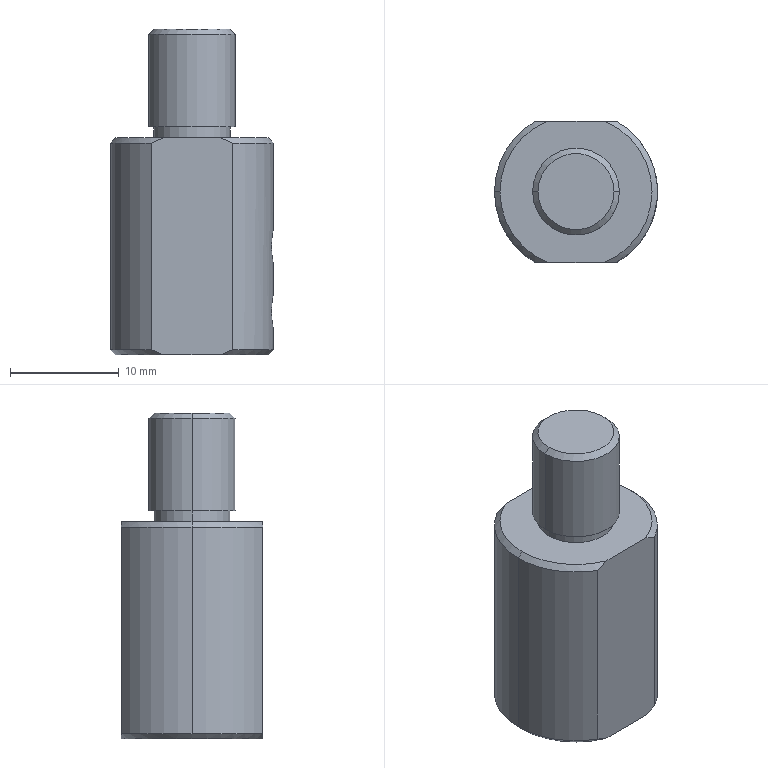Part | SolidWorks | features ICE 4, Chamfer 1, Extrusion 1, HoleWzd 1 | 1 solid | 32 faces | box 15 x 13 x 30 mm | volume 3613 mm3 | cylinder 13 | plane 11 | cone 8 | commonest cylinder face diameters 3.3 x4 15 x3 3 x2 7 x2 8 x2
STEP:
#1=CARTESIAN_POINT('',(7.5,0.,2.35));
#2=VERTEX_POINT('',#1);
#3=CARTESIAN_POINT('',(7.5,0.,5.65));
#4=VERTEX_POINT('',#3);
#5=CARTESIAN_POINT('',(7.5,0.,2.35));
#6=CARTESIAN_POINT('',(7.5,-0.2157,2.35));
#7=CARTESIAN_POINT('',(7.49,-0.4334,2.393));
#8=CARTESIAN_POINT('',(7.465,-0.7314,2.517));
#9=CARTESIAN_POINT('',(7.455,-0.8278,2.569));
#10=CARTESIAN_POINT('',(7.433,-1.007,2.689));
#11=CARTESIAN_POINT('',(7.421,-1.09,2.757));
#12=CARTESIAN_POINT('',(7.397,-1.242,2.909));
#13=CARTESIAN_POINT('',(7.385,-1.312,2.993));
#14=CARTESIAN_POINT('',(7.362,-1.431,3.172));
#15=CARTESIAN_POINT('',(7.352,-1.482,3.266));
#16=CARTESIAN_POINT('',(7.326,-1.607,3.567));
#17=CARTESIAN_POINT('',(7.316,-1.65,3.782));
#18=CARTESIAN_POINT('',(7.316,-1.65,4.108));
#19=CARTESIAN_POINT('',(7.319,-1.639,4.216));
#20=CARTESIAN_POINT('',(7.328,-1.597,4.427));
#21=CARTESIAN_POINT('',(7.335,-1.565,4.532));
#22=CARTESIAN_POINT('',(7.361,-1.442,4.831));
#23=CARTESIAN_POINT('',(7.385,-1.319,5.014));
#24=CARTESIAN_POINT('',(7.432,-1.016,5.318));
#25=CARTESIAN_POINT('',(7.456,-0.8326,5.441));
#26=CARTESIAN_POINT('',(7.482,-0.5349,5.565));
#27=CARTESIAN_POINT('',(7.488,-0.43,5.597));
#28=CARTESIAN_POINT('',(7.498,-0.2172,5.639));
#29=CARTESIAN_POINT('',(7.5,-0.1094,5.65));
#30=CARTESIAN_POINT('',(7.5,0.,5.65));
#31=B_SPLINE_CURVE_WITH_KNOTS('',3,(#5,#6,#7,#8,#9,#10,#11,#12,#13,#14,#15,#16,#17,#18,#19,#20,#21,#22,#23,#24,#25,#26,#27,#28,#29,#30),.UNSPECIFIED.,.F.,.F.,(4,2,2,2,2,2,2,2,2,2,2,2,4),(0.005175,0.005821,0.006144,0.006468,0.006791,0.007114,0.007761,0.008084,0.008408,0.009054,0.009701,0.01002,0.01035),.UNSPECIFIED.);
#32=EDGE_CURVE('',#2,#4,#31,.T.);
#33=ORIENTED_EDGE('',*,*,#32,.F.);
#34=CARTESIAN_POINT('',(1.5,0.,2.35));
#35=VERTEX_POINT('',#34);
#36=CARTESIAN_POINT('',(0.,0.,2.35));
#37=DIRECTION('',(-1.,0.,0.));
#38=VECTOR('',#37,1000.);
#39=LINE('',#36,#38);
#40=EDGE_CURVE('',#2,#35,#39,.T.);
#41=ORIENTED_EDGE('',*,*,#40,.T.);
#42=CARTESIAN_POINT('',(0.,-1.5,3.313));
#43=VERTEX_POINT('',#42);
#44=CARTESIAN_POINT('',(0.,-1.5,3.313));
#45=CARTESIAN_POINT('',(0.1094,-1.5,3.313));
#46=CARTESIAN_POINT('',(0.2147,-1.488,3.285));
#47=CARTESIAN_POINT('',(0.4105,-1.446,3.204));
#48=CARTESIAN_POINT('',(0.5002,-1.417,3.152));
#49=CARTESIAN_POINT('',(0.7569,-1.308,2.986));
#50=CARTESIAN_POINT('',(0.9049,-1.21,2.866));
#51=CARTESIAN_POINT('',(1.172,-0.9546,2.644));
#52=CARTESIAN_POINT('',(1.286,-0.798,2.542));
#53=CARTESIAN_POINT('',(1.411,-0.5202,2.431));
#54=CARTESIAN_POINT('',(1.443,-0.4223,2.401));
#55=CARTESIAN_POINT('',(1.488,-0.2144,2.361));
#56=CARTESIAN_POINT('',(1.5,-0.1072,2.35));
#57=CARTESIAN_POINT('',(1.5,0.,2.35));
#58=B_SPLINE_CURVE_WITH_KNOTS('',3,(#44,#45,#46,#47,#48,#49,#50,#51,#52,#53,#54,#55,#56,#57),.UNSPECIFIED.,.F.,.F.,(4,2,2,2,2,2,4),(0.,0.000322,0.000644,0.001288,0.001932,0.002254,0.002576),.UNSPECIFIED.);
#59=EDGE_CURVE('',#43,#35,#58,.T.);
#60=ORIENTED_EDGE('',*,*,#59,.F.);
#61=CARTESIAN_POINT('',(0.,-1.5,4.687));
#62=VERTEX_POINT('',#61);
#63=CARTESIAN_POINT('',(0.,0.,4.));
#64=DIRECTION('',(-1.,0.,0.));
#65=DIRECTION('',(0.,0.,1.));
#66=AXIS2_PLACEMENT_3D('',#63,#64,#65);
#67=CIRCLE('',#66,1.65);
#68=EDGE_CURVE('',#43,#62,#67,.T.);
#69=ORIENTED_EDGE('',*,*,#68,.T.);
#70=CARTESIAN_POINT('',(1.5,0.,5.65));
#71=VERTEX_POINT('',#70);
#72=CARTESIAN_POINT('',(1.5,0.,5.65));
#73=CARTESIAN_POINT('',(1.5,-0.107,5.65));
#74=CARTESIAN_POINT('',(1.488,-0.2158,5.639));
#75=CARTESIAN_POINT('',(1.443,-0.4216,5.599));
#76=CARTESIAN_POINT('',(1.41,-0.5214,5.569));
#77=CARTESIAN_POINT('',(1.286,-0.7979,5.458));
#78=CARTESIAN_POINT('',(1.171,-0.9551,5.356));
#79=CARTESIAN_POINT('',(0.9067,-1.209,5.135));
#80=CARTESIAN_POINT('',(0.7555,-1.309,5.013));
#81=CARTESIAN_POINT('',(0.5018,-1.417,4.849));
#82=CARTESIAN_POINT('',(0.4108,-1.446,4.796));
#83=CARTESIAN_POINT('',(0.2156,-1.488,4.715));
#84=CARTESIAN_POINT('',(0.1091,-1.5,4.687));
#85=CARTESIAN_POINT('',(0.,-1.5,4.687));
#86=B_SPLINE_CURVE_WITH_KNOTS('',3,(#72,#73,#74,#75,#76,#77,#78,#79,#80,#81,#82,#83,#84,#85),.UNSPECIFIED.,.F.,.F.,(4,2,2,2,2,2,4),(0.002576,0.002897,0.003219,0.003861,0.004504,0.004825,0.005146),.UNSPECIFIED.);
#87=EDGE_CURVE('',#71,#62,#86,.T.);
#88=ORIENTED_EDGE('',*,*,#87,.F.);
#89=CARTESIAN_POINT('',(0.,0.,5.65));
#90=DIRECTION('',(-1.,0.,0.));
#91=VECTOR('',#90,1000.);
#92=LINE('',#89,#91);
#93=EDGE_CURVE('',#4,#71,#92,.T.);
#94=ORIENTED_EDGE('',*,*,#93,.F.);
#95=EDGE_LOOP('',(#33,#41,#60,#69,#88,#94));
#96=FACE_OUTER_BOUND('',#95,.T.);
#97=CARTESIAN_POINT('',(0.,0.,4.));
#98=DIRECTION('',(-1.,0.,0.));
#99=DIRECTION('',(0.,0.,1.));
#100=AXIS2_PLACEMENT_3D('',#97,#98,#99);
#101=CYLINDRICAL_SURFACE('',#100,1.65);
#102=ADVANCED_FACE('',(#96),#101,.F.);
#103=CARTESIAN_POINT('',(7.5,0.,8.35));
#104=VERTEX_POINT('',#103);
#105=CARTESIAN_POINT('',(7.5,0.,11.65));
#106=VERTEX_POINT('',#105);
#107=CARTESIAN_POINT('',(7.5,0.,8.35));
#108=CARTESIAN_POINT('',(7.5,-0.2157,8.35));
#109=CARTESIAN_POINT('',(7.49,-0.4334,8.393));
#110=CARTESIAN_POINT('',(7.465,-0.7314,8.517));
#111=CARTESIAN_POINT('',(7.455,-0.8278,8.569));
#112=CARTESIAN_POINT('',(7.433,-1.007,8.689));
#113=CARTESIAN_POINT('',(7.421,-1.09,8.757));
#114=CARTESIAN_POINT('',(7.397,-1.242,8.909));
#115=CARTESIAN_POINT('',(7.385,-1.312,8.993));
#116=CARTESIAN_POINT('',(7.362,-1.431,9.172));
#117=CARTESIAN_POINT('',(7.352,-1.482,9.266));
#118=CARTESIAN_POINT('',(7.326,-1.607,9.567));
#119=CARTESIAN_POINT('',(7.316,-1.65,9.782));
#120=CARTESIAN_POINT('',(7.316,-1.65,10.108));
#121=CARTESIAN_POINT('',(7.319,-1.639,10.216));
#122=CARTESIAN_POINT('',(7.328,-1.597,10.427));
#123=CARTESIAN_POINT('',(7.335,-1.565,10.532));
#124=CARTESIAN_POINT('',(7.361,-1.442,10.831));
#125=CARTESIAN_POINT('',(7.385,-1.319,11.014));
#126=CARTESIAN_POINT('',(7.432,-1.016,11.318));
#127=CARTESIAN_POINT('',(7.456,-0.8326,11.441));
#128=CARTESIAN_POINT('',(7.482,-0.5349,11.565));
#129=CARTESIAN_POINT('',(7.488,-0.43,11.597));
#130=CARTESIAN_POINT('',(7.498,-0.2172,11.639));
#131=CARTESIAN_POINT('',(7.5,-0.1094,11.65));
#132=CARTESIAN_POINT('',(7.5,0.,11.65));
#133=B_SPLINE_CURVE_WITH_KNOTS('',3,(#107,#108,#109,#110,#111,#112,#113,#114,#115,#116,#117,#118,#119,#120,#121,#122,#123,#124,#125,#126,#127,#128,#129,#130,#131,#132),.UNSPECIFIED.,.F.,.F.,(4,2,2,2,2,2,2,2,2,2,2,2,4),(0.005175,0.005821,0.006144,0.006468,0.006791,0.007114,0.007761,0.008084,0.008408,0.009054,0.009701,0.01002,0.01035),.UNSPECIFIED.);
#134=EDGE_CURVE('',#104,#106,#133,.T.);
#135=ORIENTED_EDGE('',*,*,#134,.F.);
#136=CARTESIAN_POINT('',(1.5,0.,8.35));
#137=VERTEX_POINT('',#136);
#138=CARTESIAN_POINT('',(0.,0.,8.35));
#139=DIRECTION('',(-1.,0.,0.));
#140=VECTOR('',#139,1000.);
#141=LINE('',#138,#140);
#142=EDGE_CURVE('',#104,#137,#141,.T.);
#143=ORIENTED_EDGE('',*,*,#142,.T.);
#144=CARTESIAN_POINT('',(0.,-1.5,9.313));
#145=VERTEX_POINT('',#144);
#146=CARTESIAN_POINT('',(0.,-1.5,9.313));
#147=CARTESIAN_POINT('',(0.1094,-1.5,9.313));
#148=CARTESIAN_POINT('',(0.2147,-1.488,9.285));
#149=CARTESIAN_POINT('',(0.4105,-1.446,9.204));
#150=CARTESIAN_POINT('',(0.5002,-1.417,9.152));
#151=CARTESIAN_POINT('',(0.7569,-1.308,8.986));
#152=CARTESIAN_POINT('',(0.9049,-1.21,8.866));
#153=CARTESIAN_POINT('',(1.172,-0.9546,8.644));
#154=CARTESIAN_POINT('',(1.286,-0.798,8.542));
#155=CARTESIAN_POINT('',(1.411,-0.5202,8.431));
#156=CARTESIAN_POINT('',(1.443,-0.4223,8.401));
#157=CARTESIAN_POINT('',(1.488,-0.2144,8.361));
#158=CARTESIAN_POINT('',(1.5,-0.1072,8.35));
#159=CARTESIAN_POINT('',(1.5,0.,8.35));
#160=B_SPLINE_CURVE_WITH_KNOTS('',3,(#146,#147,#148,#149,#150,#151,#152,#153,#154,#155,#156,#157,#158,#159),.UNSPECIFIED.,.F.,.F.,(4,2,2,2,2,2,4),(0.,0.000322,0.000644,0.001288,0.001932,0.002254,0.002576),.UNSPECIFIED.);
#161=EDGE_CURVE('',#145,#137,#160,.T.);
#162=ORIENTED_EDGE('',*,*,#161,.F.);
#163=CARTESIAN_POINT('',(0.,-1.5,10.687));
#164=VERTEX_POINT('',#163);
#165=CARTESIAN_POINT('',(0.,0.,10.));
#166=DIRECTION('',(-1.,0.,0.));
#167=DIRECTION('',(0.,0.,1.));
#168=AXIS2_PLACEMENT_3D('',#165,#166,#167);
#169=CIRCLE('',#168,1.65);
#170=EDGE_CURVE('',#145,#164,#169,.T.);
#171=ORIENTED_EDGE('',*,*,#170,.T.);
#172=CARTESIAN_POINT('',(1.5,0.,11.65));
#173=VERTEX_POINT('',#172);
#174=CARTESIAN_POINT('',(1.5,0.,11.65));
#175=CARTESIAN_POINT('',(1.5,-0.107,11.65));
#176=CARTESIAN_POINT('',(1.488,-0.2158,11.639));
#177=CARTESIAN_POINT('',(1.443,-0.4216,11.599));
#178=CARTESIAN_POINT('',(1.41,-0.5214,11.569));
#179=CARTESIAN_POINT('',(1.286,-0.7979,11.458));
#180=CARTESIAN_POINT('',(1.171,-0.9551,11.356));
#181=CARTESIAN_POINT('',(0.9067,-1.209,11.135));
#182=CARTESIAN_POINT('',(0.7555,-1.309,11.013));
#183=CARTESIAN_POINT('',(0.5018,-1.417,10.849));
#184=CARTESIAN_POINT('',(0.4108,-1.446,10.796));
#185=CARTESIAN_POINT('',(0.2156,-1.488,10.715));
#186=CARTESIAN_POINT('',(0.1091,-1.5,10.687));
#187=CARTESIAN_POINT('',(0.,-1.5,10.687));
#188=B_SPLINE_CURVE_WITH_KNOTS('',3,(#174,#175,#176,#177,#178,#179,#180,#181,#182,#183,#184,#185,#186,#187),.UNSPECIFIED.,.F.,.F.,(4,2,2,2,2,2,4),(0.002576,0.002897,0.003219,0.003861,0.004504,0.004825,0.005146),.UNSPECIFIED.);
#189=EDGE_CURVE('',#173,#164,#188,.T.);
#190=ORIENTED_EDGE('',*,*,#189,.F.);
#191=CARTESIAN_POINT('',(0.,0.,11.65));
#192=DIRECTION('',(-1.,0.,0.));
#193=VECTOR('',#192,1000.);
#194=LINE('',#191,#193);
#195=EDGE_CURVE('',#106,#173,#194,.T.);
#196=ORIENTED_EDGE('',*,*,#195,.F.);
#197=EDGE_LOOP('',(#135,#143,#162,#171,#190,#196));
#198=FACE_OUTER_BOUND('',#197,.T.);
#199=CARTESIAN_POINT('',(0.,0.,10.));
#200=DIRECTION('',(-1.,0.,0.));
#201=DIRECTION('',(0.,0.,1.));
#202=AXIS2_PLACEMENT_3D('',#199,#200,#201);
#203=CYLINDRICAL_SURFACE('',#202,1.65);
#204=ADVANCED_FACE('',(#198),#203,.F.);
#205=CARTESIAN_POINT('',(7.,0.,0.));
#206=VERTEX_POINT('',#205);
#207=CARTESIAN_POINT('',(2.598,-6.5,0.));
#208=VERTEX_POINT('',#207);
#209=CARTESIAN_POINT('',(0.,0.,0.));
#210=DIRECTION('',(0.,0.,-1.));
#211=DIRECTION('',(1.,0.,0.));
#212=AXIS2_PLACEMENT_3D('',#209,#210,#211);
#213=CIRCLE('',#212,7.);
#214=EDGE_CURVE('',#206,#208,#213,.T.);
#215=ORIENTED_EDGE('',*,*,#214,.F.);
#216=CARTESIAN_POINT('',(7.5,0.,0.5));
#217=VERTEX_POINT('',#216);
#218=CARTESIAN_POINT('',(7.5,0.,0.5));
#219=DIRECTION('',(0.7071,0.,0.7071));
#220=VECTOR('',#219,1000.);
#221=LINE('',#218,#220);
#222=EDGE_CURVE('',#206,#217,#221,.T.);
#223=ORIENTED_EDGE('',*,*,#222,.T.);
#224=CARTESIAN_POINT('',(3.742,-6.5,0.5));
#225=VERTEX_POINT('',#224);
#226=CARTESIAN_POINT('',(0.,0.,0.5));
#227=DIRECTION('',(0.,0.,1.));
#228=DIRECTION('',(1.,0.,0.));
#229=AXIS2_PLACEMENT_3D('',#226,#227,#228);
#230=CIRCLE('',#229,7.5);
#231=EDGE_CURVE('',#225,#217,#230,.T.);
#232=ORIENTED_EDGE('',*,*,#231,.F.);
#233=CARTESIAN_POINT('',(2.598,-6.5,0.));
#234=CARTESIAN_POINT('',(2.988,-6.5,0.1448));
#235=CARTESIAN_POINT('',(3.371,-6.5,0.3152));
#236=CARTESIAN_POINT('',(3.742,-6.5,0.5));
#237=B_SPLINE_CURVE_WITH_KNOTS('',3,(#233,#234,#235,#236),.UNSPECIFIED.,.F.,.F.,(4,4),(0.01557,0.01681),.UNSPECIFIED.);
#238=EDGE_CURVE('',#208,#225,#237,.T.);
#239=ORIENTED_EDGE('',*,*,#238,.F.);
#240=EDGE_LOOP('',(#215,#223,#232,#239));
#241=FACE_OUTER_BOUND('',#240,.T.);
#242=CARTESIAN_POINT('',(0.,0.,0.5));
#243=DIRECTION('',(0.,0.,1.));
#244=DIRECTION('',(1.,0.,0.));
#245=AXIS2_PLACEMENT_3D('',#242,#243,#244);
#246=CONICAL_SURFACE('',#245,7.5,0.7854);
#247=ADVANCED_FACE('',(#241),#246,.T.);
#248=CARTESIAN_POINT('',(-7.,0.,20.));
#249=VERTEX_POINT('',#248);
#250=CARTESIAN_POINT('',(-2.598,-6.5,20.));
#251=VERTEX_POINT('',#250);
#252=CARTESIAN_POINT('',(0.,0.,20.));
#253=DIRECTION('',(0.,0.,1.));
#254=DIRECTION('',(1.,0.,0.));
#255=AXIS2_PLACEMENT_3D('',#252,#253,#254);
#256=CIRCLE('',#255,7.);
#257=EDGE_CURVE('',#249,#251,#256,.T.);
#258=ORIENTED_EDGE('',*,*,#257,.F.);
#259=CARTESIAN_POINT('',(-7.5,0.,19.5));
#260=VERTEX_POINT('',#259);
#261=CARTESIAN_POINT('',(-7.,0.,20.));
#262=DIRECTION('',(-0.7071,0.,-0.7071));
#263=VECTOR('',#262,1000.);
#264=LINE('',#261,#263);
#265=EDGE_CURVE('',#249,#260,#264,.T.);
#266=ORIENTED_EDGE('',*,*,#265,.T.);
#267=CARTESIAN_POINT('',(-3.742,-6.5,19.5));
#268=VERTEX_POINT('',#267);
#269=CARTESIAN_POINT('',(0.,0.,19.5));
#270=DIRECTION('',(0.,0.,-1.));
#271=DIRECTION('',(1.,0.,0.));
#272=AXIS2_PLACEMENT_3D('',#269,#270,#271);
#273=CIRCLE('',#272,7.5);
#274=EDGE_CURVE('',#268,#260,#273,.T.);
#275=ORIENTED_EDGE('',*,*,#274,.F.);
#276=CARTESIAN_POINT('',(-2.598,-6.5,20.));
#277=CARTESIAN_POINT('',(-2.988,-6.5,19.855));
#278=CARTESIAN_POINT('',(-3.371,-6.5,19.685));
#279=CARTESIAN_POINT('',(-3.742,-6.5,19.5));
#280=B_SPLINE_CURVE_WITH_KNOTS('',3,(#276,#277,#278,#279),.UNSPECIFIED.,.F.,.F.,(4,4),(0.01557,0.01681),.UNSPECIFIED.);
#281=EDGE_CURVE('',#251,#268,#280,.T.);
#282=ORIENTED_EDGE('',*,*,#281,.F.);
#283=EDGE_LOOP('',(#258,#266,#275,#282));
#284=FACE_OUTER_BOUND('',#283,.T.);
#285=CARTESIAN_POINT('',(0.,0.,20.));
#286=DIRECTION('',(0.,0.,-1.));
#287=DIRECTION('',(-1.,0.,0.));
#288=AXIS2_PLACEMENT_3D('',#285,#286,#287);
#289=CONICAL_SURFACE('',#288,7.,0.7854);
#290=ADVANCED_FACE('',(#284),#289,.T.);
#291=CARTESIAN_POINT('',(3.5,0.,30.));
#292=VERTEX_POINT('',#291);
#293=CARTESIAN_POINT('',(-3.5,0.,30.));
#294=VERTEX_POINT('',#293);
#295=CARTESIAN_POINT('',(0.,0.,30.));
#296=DIRECTION('',(0.,0.,1.));
#297=DIRECTION('',(1.,0.,0.));
#298=AXIS2_PLACEMENT_3D('',#295,#296,#297);
#299=CIRCLE('',#298,3.5);
#300=EDGE_CURVE('',#292,#294,#299,.T.);
#301=ORIENTED_EDGE('',*,*,#300,.F.);
#302=CARTESIAN_POINT('',(4.,0.,29.5));
#303=VERTEX_POINT('',#302);
#304=CARTESIAN_POINT('',(3.5,0.,30.));
#305=DIRECTION('',(0.7071,0.,-0.7071));
#306=VECTOR('',#305,1000.);
#307=LINE('',#304,#306);
#308=EDGE_CURVE('',#292,#303,#307,.T.);
#309=ORIENTED_EDGE('',*,*,#308,.T.);
#310=CARTESIAN_POINT('',(-4.,0.,29.5));
#311=VERTEX_POINT('',#310);
#312=CARTESIAN_POINT('',(0.,0.,29.5));
#313=DIRECTION('',(0.,0.,-1.));
#314=DIRECTION('',(1.,0.,0.));
#315=AXIS2_PLACEMENT_3D('',#312,#313,#314);
#316=CIRCLE('',#315,4.);
#317=EDGE_CURVE('',#311,#303,#316,.T.);
#318=ORIENTED_EDGE('',*,*,#317,.F.);
#319=CARTESIAN_POINT('',(-3.5,0.,30.));
#320=DIRECTION('',(-0.7071,0.,-0.7071));
#321=VECTOR('',#320,1000.);
#322=LINE('',#319,#321);
#323=EDGE_CURVE('',#294,#311,#322,.T.);
#324=ORIENTED_EDGE('',*,*,#323,.F.);
#325=EDGE_LOOP('',(#301,#309,#318,#324));
#326=FACE_OUTER_BOUND('',#325,.T.);
#327=CARTESIAN_POINT('',(0.,0.,30.));
#328=DIRECTION('',(0.,0.,-1.));
#329=DIRECTION('',(-1.,0.,0.));
#330=AXIS2_PLACEMENT_3D('',#327,#328,#329);
#331=CONICAL_SURFACE('',#330,3.5,0.7854);
#332=ADVANCED_FACE('',(#326),#331,.T.);
#333=CARTESIAN_POINT('',(-4.,0.,21.));
#334=VERTEX_POINT('',#333);
#335=CARTESIAN_POINT('',(4.,0.,21.));
#336=VERTEX_POINT('',#335);
#337=CARTESIAN_POINT('',(0.,0.,21.));
#338=DIRECTION('',(0.,0.,-1.));
#339=DIRECTION('',(1.,0.,0.));
#340=AXIS2_PLACEMENT_3D('',#337,#338,#339);
#341=CIRCLE('',#340,4.);
#342=EDGE_CURVE('',#334,#336,#341,.T.);
#343=ORIENTED_EDGE('',*,*,#342,.F.);
#344=CARTESIAN_POINT('',(-4.,0.,20.));
#345=DIRECTION('',(0.,0.,1.));
#346=VECTOR('',#345,1000.);
#347=LINE('',#344,#346);
#348=EDGE_CURVE('',#334,#311,#347,.T.);
#349=ORIENTED_EDGE('',*,*,#348,.T.);
#350=ORIENTED_EDGE('',*,*,#317,.T.);
#351=CARTESIAN_POINT('',(4.,0.,20.));
#352=DIRECTION('',(0.,0.,1.));
#353=VECTOR('',#352,1000.);
#354=LINE('',#351,#353);
#355=EDGE_CURVE('',#336,#303,#354,.T.);
#356=ORIENTED_EDGE('',*,*,#355,.F.);
#357=EDGE_LOOP('',(#343,#349,#350,#356));
#358=FACE_OUTER_BOUND('',#357,.T.);
#359=CARTESIAN_POINT('',(0.,0.,20.));
#360=DIRECTION('',(0.,0.,1.));
#361=DIRECTION('',(1.,0.,0.));
#362=AXIS2_PLACEMENT_3D('',#359,#360,#361);
#363=CYLINDRICAL_SURFACE('',#362,4.);
#364=ADVANCED_FACE('',(#358),#363,.T.);
#365=CARTESIAN_POINT('',(3.5,0.,21.));
#366=VERTEX_POINT('',#365);
#367=CARTESIAN_POINT('',(-3.5,0.,21.));
#368=VERTEX_POINT('',#367);
#369=CARTESIAN_POINT('',(0.,0.,21.));
#370=DIRECTION('',(0.,0.,1.));
#371=DIRECTION('',(1.,0.,0.));
#372=AXIS2_PLACEMENT_3D('',#369,#370,#371);
#373=CIRCLE('',#372,3.5);
#374=EDGE_CURVE('',#366,#368,#373,.T.);
#375=ORIENTED_EDGE('',*,*,#374,.F.);
#376=CARTESIAN_POINT('',(3.5,0.,20.));
#377=VERTEX_POINT('',#376);
#378=CARTESIAN_POINT('',(3.5,0.,21.));
#379=DIRECTION('',(0.,0.,-1.));
#380=VECTOR('',#379,1000.);
#381=LINE('',#378,#380);
#382=EDGE_CURVE('',#366,#377,#381,.T.);
#383=ORIENTED_EDGE('',*,*,#382,.T.);
#384=CARTESIAN_POINT('',(-3.5,0.,20.));
#385=VERTEX_POINT('',#384);
#386=CARTESIAN_POINT('',(0.,0.,20.));
#387=DIRECTION('',(0.,0.,1.));
#388=DIRECTION('',(1.,0.,0.));
#389=AXIS2_PLACEMENT_3D('',#386,#387,#388);
#390=CIRCLE('',#389,3.5);
#391=EDGE_CURVE('',#377,#385,#390,.T.);
#392=ORIENTED_EDGE('',*,*,#391,.T.);
#393=CARTESIAN_POINT('',(-3.5,0.,21.));
#394=DIRECTION('',(0.,0.,-1.));
#395=VECTOR('',#394,1000.);
#396=LINE('',#393,#395);
#397=EDGE_CURVE('',#368,#385,#396,.T.);
#398=ORIENTED_EDGE('',*,*,#397,.F.);
#399=EDGE_LOOP('',(#375,#383,#392,#398));
#400=FACE_OUTER_BOUND('',#399,.T.);
#401=CARTESIAN_POINT('',(0.,0.,21.));
#402=DIRECTION('',(0.,0.,-1.));
#403=DIRECTION('',(-1.,0.,0.));
#404=AXIS2_PLACEMENT_3D('',#401,#402,#403);
#405=CYLINDRICAL_SURFACE('',#404,3.5);
#406=ADVANCED_FACE('',(#400),#405,.T.);
#407=CARTESIAN_POINT('',(1.5,0.,13.));
#408=VERTEX_POINT('',#407);
#409=CARTESIAN_POINT('',(-1.5,0.,13.));
#410=VERTEX_POINT('',#409);
#411=CARTESIAN_POINT('',(0.,0.,13.));
#412=DIRECTION('',(0.,0.,-1.));
#413=DIRECTION('',(-1.,0.,0.));
#414=AXIS2_PLACEMENT_3D('',#411,#412,#413);
#415=CIRCLE('',#414,1.5);
#416=EDGE_CURVE('',#408,#410,#415,.T.);
#417=ORIENTED_EDGE('',*,*,#416,.F.);
#418=CARTESIAN_POINT('',(1.5,0.,13.));
#419=DIRECTION('',(0.,0.,-1.));
#420=VECTOR('',#419,1000.);
#421=LINE('',#418,#420);
#422=EDGE_CURVE('',#408,#173,#421,.T.);
#423=ORIENTED_EDGE('',*,*,#422,.T.);
#424=ORIENTED_EDGE('',*,*,#189,.T.);
#425=CARTESIAN_POINT('',(0.,-1.5,13.));
#426=DIRECTION('',(0.,0.,-1.));
#427=VECTOR('',#426,1000.);
#428=LINE('',#425,#427);
#429=EDGE_CURVE('',#164,#145,#428,.T.);
#430=ORIENTED_EDGE('',*,*,#429,.T.);
#431=ORIENTED_EDGE('',*,*,#161,.T.);
#432=CARTESIAN_POINT('',(1.5,0.,13.));
#433=DIRECTION('',(0.,0.,-1.));
#434=VECTOR('',#433,1000.);
#435=LINE('',#432,#434);
#436=EDGE_CURVE('',#137,#71,#435,.T.);
#437=ORIENTED_EDGE('',*,*,#436,.T.);
#438=ORIENTED_EDGE('',*,*,#87,.T.);
#439=CARTESIAN_POINT('',(0.,-1.5,13.));
#440=DIRECTION('',(0.,0.,-1.));
#441=VECTOR('',#440,1000.);
#442=LINE('',#439,#441);
#443=EDGE_CURVE('',#62,#43,#442,.T.);
#444=ORIENTED_EDGE('',*,*,#443,.T.);
#445=ORIENTED_EDGE('',*,*,#59,.T.);
#446=CARTESIAN_POINT('',(1.5,0.,0.));
#447=VERTEX_POINT('',#446);
#448=CARTESIAN_POINT('',(1.5,0.,13.));
#449=DIRECTION('',(0.,0.,-1.));
#450=VECTOR('',#449,1000.);
#451=LINE('',#448,#450);
#452=EDGE_CURVE('',#35,#447,#451,.T.);
#453=ORIENTED_EDGE('',*,*,#452,.T.);
#454=CARTESIAN_POINT('',(-1.5,0.,0.));
#455=VERTEX_POINT('',#454);
#456=CARTESIAN_POINT('',(0.,0.,0.));
#457=DIRECTION('',(0.,0.,-1.));
#458=DIRECTION('',(-1.,0.,0.));
#459=AXIS2_PLACEMENT_3D('',#456,#457,#458);
#460=CIRCLE('',#459,1.5);
#461=EDGE_CURVE('',#447,#455,#460,.T.);
#462=ORIENTED_EDGE('',*,*,#461,.T.);
#463=CARTESIAN_POINT('',(-1.5,0.,13.));
#464=DIRECTION('',(0.,0.,-1.));
#465=VECTOR('',#464,1000.);
#466=LINE('',#463,#465);
#467=EDGE_CURVE('',#410,#455,#466,.T.);
#468=ORIENTED_EDGE('',*,*,#467,.F.);
#469=EDGE_LOOP('',(#417,#423,#424,#430,#431,#437,#438,#444,#445,#453,#462,#468));
#470=FACE_OUTER_BOUND('',#469,.T.);
#471=CARTESIAN_POINT('',(0.,0.,13.));
#472=DIRECTION('',(0.,0.,-1.));
#473=DIRECTION('',(-1.,0.,0.));
#474=AXIS2_PLACEMENT_3D('',#471,#472,#473);
#475=CYLINDRICAL_SURFACE('',#474,1.5);
#476=ADVANCED_FACE('',(#470),#475,.F.);
#477=ORIENTED_EDGE('',*,*,#274,.T.);
#478=CARTESIAN_POINT('',(-7.5,0.,0.5));
#479=VERTEX_POINT('',#478);
#480=CARTESIAN_POINT('',(-7.5,0.,30.));
#481=DIRECTION('',(0.,0.,-1.));
#482=VECTOR('',#481,1000.);
#483=LINE('',#480,#482);
#484=EDGE_CURVE('',#260,#479,#483,.T.);
#485=ORIENTED_EDGE('',*,*,#484,.T.);
#486=CARTESIAN_POINT('',(-3.742,-6.5,0.5));
#487=VERTEX_POINT('',#486);
#488=CARTESIAN_POINT('',(0.,0.,0.5));
#489=DIRECTION('',(0.,0.,1.));
#490=DIRECTION('',(1.,0.,0.));
#491=AXIS2_PLACEMENT_3D('',#488,#489,#490);
#492=CIRCLE('',#491,7.5);
#493=EDGE_CURVE('',#479,#487,#492,.T.);
#494=ORIENTED_EDGE('',*,*,#493,.T.);
#495=CARTESIAN_POINT('',(-3.742,-6.5,30.));
#496=DIRECTION('',(0.,0.,1.));
#497=VECTOR('',#496,1000.);
#498=LINE('',#495,#497);
#499=EDGE_CURVE('',#487,#268,#498,.T.);
#500=ORIENTED_EDGE('',*,*,#499,.T.);
#501=EDGE_LOOP('',(#477,#485,#494,#500));
#502=FACE_OUTER_BOUND('',#501,.T.);
#503=CARTESIAN_POINT('',(0.,0.,30.));
#504=DIRECTION('',(0.,0.,-1.));
#505=DIRECTION('',(-1.,0.,0.));
#506=AXIS2_PLACEMENT_3D('',#503,#504,#505);
#507=CYLINDRICAL_SURFACE('',#506,7.5);
#508=ADVANCED_FACE('',(#502),#507,.T.);
#509=CARTESIAN_POINT('',(7.5,0.,11.65));
#510=CARTESIAN_POINT('',(7.5,0.1094,11.65));
#511=CARTESIAN_POINT('',(7.498,0.2169,11.639));
#512=CARTESIAN_POINT('',(7.489,0.4282,11.597));
#513=CARTESIAN_POINT('',(7.482,0.5332,11.565));
#514=CARTESIAN_POINT('',(7.465,0.7329,11.482));
#515=CARTESIAN_POINT('',(7.455,0.8275,11.432));
#516=CARTESIAN_POINT('',(7.433,1.007,11.312));
#517=CARTESIAN_POINT('',(7.421,1.091,11.242));
#518=CARTESIAN_POINT('',(7.385,1.319,11.015));
#519=CARTESIAN_POINT('',(7.361,1.442,10.831));
#520=CARTESIAN_POINT('',(7.326,1.606,10.434));
#521=CARTESIAN_POINT('',(7.316,1.65,10.217));
#522=CARTESIAN_POINT('',(7.316,1.65,9.893));
#523=CARTESIAN_POINT('',(7.319,1.639,9.783));
#524=CARTESIAN_POINT('',(7.328,1.597,9.571));
#525=CARTESIAN_POINT('',(7.335,1.566,9.468));
#526=CARTESIAN_POINT('',(7.361,1.441,9.168));
#527=CARTESIAN_POINT('',(7.385,1.32,8.986));
#528=CARTESIAN_POINT('',(7.421,1.09,8.757));
#529=CARTESIAN_POINT('',(7.433,1.007,8.689));
#530=CARTESIAN_POINT('',(7.455,0.8286,8.569));
#531=CARTESIAN_POINT('',(7.465,0.7319,8.517));
#532=CARTESIAN_POINT('',(7.482,0.5325,8.435));
#533=CARTESIAN_POINT('',(7.488,0.4297,8.403));
#534=CARTESIAN_POINT('',(7.498,0.2174,8.361));
#535=CARTESIAN_POINT('',(7.5,0.1079,8.35));
#536=CARTESIAN_POINT('',(7.5,0.,8.35));
#537=B_SPLINE_CURVE_WITH_KNOTS('',3,(#509,#510,#511,#512,#513,#514,#515,#516,#517,#518,#519,#520,#521,#522,#523,#524,#525,#526,#527,#528,#529,#530,#531,#532,#533,#534,#535,#536),.UNSPECIFIED.,.F.,.F.,(4,2,2,2,2,2,2,2,2,2,2,2,2,4),(0.,0.0003234,0.0006468,0.0009702,0.001294,0.00194,0.002587,0.002911,0.003234,0.003881,0.004204,0.004528,0.004851,0.005175),.UNSPECIFIED.);
#538=EDGE_CURVE('',#106,#104,#537,.T.);
#539=ORIENTED_EDGE('',*,*,#538,.T.);
#540=ORIENTED_EDGE('',*,*,#134,.T.);
#541=EDGE_LOOP('',(#539,#540));
#542=FACE_BOUND('',#541,.T.);
#543=CARTESIAN_POINT('',(7.5,0.,5.65));
#544=CARTESIAN_POINT('',(7.5,0.1094,5.65));
#545=CARTESIAN_POINT('',(7.498,0.2169,5.639));
#546=CARTESIAN_POINT('',(7.489,0.4282,5.597));
#547=CARTESIAN_POINT('',(7.482,0.5332,5.565));
#548=CARTESIAN_POINT('',(7.465,0.7329,5.482));
#549=CARTESIAN_POINT('',(7.455,0.8275,5.432));
#550=CARTESIAN_POINT('',(7.433,1.007,5.312));
#551=CARTESIAN_POINT('',(7.421,1.091,5.242));
#552=CARTESIAN_POINT('',(7.385,1.319,5.015));
#553=CARTESIAN_POINT('',(7.361,1.442,4.831));
#554=CARTESIAN_POINT('',(7.326,1.606,4.434));
#555=CARTESIAN_POINT('',(7.316,1.65,4.217));
#556=CARTESIAN_POINT('',(7.316,1.65,3.893));
#557=CARTESIAN_POINT('',(7.319,1.639,3.783));
#558=CARTESIAN_POINT('',(7.328,1.597,3.571));
#559=CARTESIAN_POINT('',(7.335,1.566,3.468));
#560=CARTESIAN_POINT('',(7.361,1.441,3.168));
#561=CARTESIAN_POINT('',(7.385,1.32,2.986));
#562=CARTESIAN_POINT('',(7.421,1.09,2.757));
#563=CARTESIAN_POINT('',(7.433,1.007,2.689));
#564=CARTESIAN_POINT('',(7.455,0.8286,2.569));
#565=CARTESIAN_POINT('',(7.465,0.7319,2.517));
#566=CARTESIAN_POINT('',(7.482,0.5325,2.435));
#567=CARTESIAN_POINT('',(7.488,0.4297,2.403));
#568=CARTESIAN_POINT('',(7.498,0.2174,2.361));
#569=CARTESIAN_POINT('',(7.5,0.1079,2.35));
#570=CARTESIAN_POINT('',(7.5,0.,2.35));
#571=B_SPLINE_CURVE_WITH_KNOTS('',3,(#543,#544,#545,#546,#547,#548,#549,#550,#551,#552,#553,#554,#555,#556,#557,#558,#559,#560,#561,#562,#563,#564,#565,#566,#567,#568,#569,#570),.UNSPECIFIED.,.F.,.F.,(4,2,2,2,2,2,2,2,2,2,2,2,2,4),(0.,0.0003234,0.0006468,0.0009702,0.001294,0.00194,0.002587,0.002911,0.003234,0.003881,0.004204,0.004528,0.004851,0.005175),.UNSPECIFIED.);
#572=EDGE_CURVE('',#4,#2,#571,.T.);
#573=ORIENTED_EDGE('',*,*,#572,.T.);
#574=ORIENTED_EDGE('',*,*,#32,.T.);
#575=EDGE_LOOP('',(#573,#574));
#576=FACE_BOUND('',#575,.T.);
#577=CARTESIAN_POINT('',(3.742,6.5,19.5));
#578=VERTEX_POINT('',#577);
#579=CARTESIAN_POINT('',(3.742,-6.5,19.5));
#580=VERTEX_POINT('',#579);
#581=CARTESIAN_POINT('',(0.,0.,19.5));
#582=DIRECTION('',(0.,0.,-1.));
#583=DIRECTION('',(1.,0.,0.));
#584=AXIS2_PLACEMENT_3D('',#581,#582,#583);
#585=CIRCLE('',#584,7.5);
#586=EDGE_CURVE('',#578,#580,#585,.T.);
#587=ORIENTED_EDGE('',*,*,#586,.T.);
#588=CARTESIAN_POINT('',(3.742,-6.5,30.));
#589=DIRECTION('',(0.,0.,-1.));
#590=VECTOR('',#589,1000.);
#591=LINE('',#588,#590);
#592=EDGE_CURVE('',#580,#225,#591,.T.);
#593=ORIENTED_EDGE('',*,*,#592,.T.);
#594=ORIENTED_EDGE('',*,*,#231,.T.);
#595=CARTESIAN_POINT('',(3.742,6.5,0.5));
#596=VERTEX_POINT('',#595);
#597=CARTESIAN_POINT('',(0.,0.,0.5));
#598=DIRECTION('',(0.,0.,1.));
#599=DIRECTION('',(1.,0.,0.));
#600=AXIS2_PLACEMENT_3D('',#597,#598,#599);
#601=CIRCLE('',#600,7.5);
#602=EDGE_CURVE('',#217,#596,#601,.T.);
#603=ORIENTED_EDGE('',*,*,#602,.T.);
#604=CARTESIAN_POINT('',(3.742,6.5,30.));
#605=DIRECTION('',(0.,0.,1.));
#606=VECTOR('',#605,1000.);
#607=LINE('',#604,#606);
#608=EDGE_CURVE('',#596,#578,#607,.T.);
#609=ORIENTED_EDGE('',*,*,#608,.T.);
#610=EDGE_LOOP('',(#587,#593,#594,#603,#609));
#611=FACE_OUTER_BOUND('',#610,.T.);
#612=CARTESIAN_POINT('',(0.,0.,30.));
#613=DIRECTION('',(0.,0.,-1.));
#614=DIRECTION('',(-1.,0.,0.));
#615=AXIS2_PLACEMENT_3D('',#612,#613,#614);
#616=CYLINDRICAL_SURFACE('',#615,7.5);
#617=ADVANCED_FACE('',(#542,#576,#611),#616,.T.);
#618=CARTESIAN_POINT('',(2.598,-6.5,20.));
#619=VERTEX_POINT('',#618);
#620=CARTESIAN_POINT('',(3.742,-6.5,19.5));
#621=CARTESIAN_POINT('',(3.371,-6.5,19.685));
#622=CARTESIAN_POINT('',(2.991,-6.5,19.854));
#623=CARTESIAN_POINT('',(2.598,-6.5,20.));
#624=B_SPLINE_CURVE_WITH_KNOTS('',3,(#620,#621,#622,#623),.UNSPECIFIED.,.F.,.F.,(4,4),(0.009016,0.01027),.UNSPECIFIED.);
#625=EDGE_CURVE('',#580,#619,#624,.T.);
#626=ORIENTED_EDGE('',*,*,#625,.F.);
#627=ORIENTED_EDGE('',*,*,#586,.F.);
#628=CARTESIAN_POINT('',(2.598,6.5,20.));
#629=VERTEX_POINT('',#628);
#630=CARTESIAN_POINT('',(2.598,6.5,20.));
#631=CARTESIAN_POINT('',(2.988,6.5,19.855));
#632=CARTESIAN_POINT('',(3.371,6.5,19.685));
#633=CARTESIAN_POINT('',(3.742,6.5,19.5));
#634=B_SPLINE_CURVE_WITH_KNOTS('',3,(#630,#631,#632,#633),.UNSPECIFIED.,.F.,.F.,(4,4),(0.01557,0.01681),.UNSPECIFIED.);
#635=EDGE_CURVE('',#629,#578,#634,.T.);
#636=ORIENTED_EDGE('',*,*,#635,.F.);
#637=CARTESIAN_POINT('',(0.,0.,20.));
#638=DIRECTION('',(0.,0.,1.));
#639=DIRECTION('',(1.,0.,0.));
#640=AXIS2_PLACEMENT_3D('',#637,#638,#639);
#641=CIRCLE('',#640,7.);
#642=EDGE_CURVE('',#619,#629,#641,.T.);
#643=ORIENTED_EDGE('',*,*,#642,.F.);
#644=EDGE_LOOP('',(#626,#627,#636,#643));
#645=FACE_OUTER_BOUND('',#644,.T.);
#646=CARTESIAN_POINT('',(0.,0.,20.));
#647=DIRECTION('',(0.,0.,-1.));
#648=DIRECTION('',(-1.,0.,0.));
#649=AXIS2_PLACEMENT_3D('',#646,#647,#648);
#650=CONICAL_SURFACE('',#649,7.,0.7854);
#651=ADVANCED_FACE('',(#645),#650,.T.);
#652=CARTESIAN_POINT('',(-2.598,-6.5,0.));
#653=VERTEX_POINT('',#652);
#654=CARTESIAN_POINT('',(-3.742,-6.5,0.5));
#655=CARTESIAN_POINT('',(-3.371,-6.5,0.315));
#656=CARTESIAN_POINT('',(-2.991,-6.5,0.1458));
#657=CARTESIAN_POINT('',(-2.598,-6.5,0.));
#658=B_SPLINE_CURVE_WITH_KNOTS('',3,(#654,#655,#656,#657),.UNSPECIFIED.,.F.,.F.,(4,4),(0.009016,0.01027),.UNSPECIFIED.);
#659=EDGE_CURVE('',#487,#653,#658,.T.);
#660=ORIENTED_EDGE('',*,*,#659,.F.);
#661=ORIENTED_EDGE('',*,*,#493,.F.);
#662=CARTESIAN_POINT('',(-3.742,6.5,0.5));
#663=VERTEX_POINT('',#662);
#664=CARTESIAN_POINT('',(0.,0.,0.5));
#665=DIRECTION('',(0.,0.,1.));
#666=DIRECTION('',(1.,0.,0.));
#667=AXIS2_PLACEMENT_3D('',#664,#665,#666);
#668=CIRCLE('',#667,7.5);
#669=EDGE_CURVE('',#663,#479,#668,.T.);
#670=ORIENTED_EDGE('',*,*,#669,.F.);
#671=CARTESIAN_POINT('',(-2.598,6.5,0.));
#672=VERTEX_POINT('',#671);
#673=CARTESIAN_POINT('',(-2.598,6.5,0.));
#674=CARTESIAN_POINT('',(-2.988,6.5,0.1448));
#675=CARTESIAN_POINT('',(-3.371,6.5,0.3152));
#676=CARTESIAN_POINT('',(-3.742,6.5,0.5));
#677=B_SPLINE_CURVE_WITH_KNOTS('',3,(#673,#674,#675,#676),.UNSPECIFIED.,.F.,.F.,(4,4),(0.01557,0.01681),.UNSPECIFIED.);
#678=EDGE_CURVE('',#672,#663,#677,.T.);
#679=ORIENTED_EDGE('',*,*,#678,.F.);
#680=CARTESIAN_POINT('',(0.,0.,0.));
#681=DIRECTION('',(0.,0.,-1.));
#682=DIRECTION('',(1.,0.,0.));
#683=AXIS2_PLACEMENT_3D('',#680,#681,#682);
#684=CIRCLE('',#683,7.);
#685=EDGE_CURVE('',#653,#672,#684,.T.);
#686=ORIENTED_EDGE('',*,*,#685,.F.);
#687=EDGE_LOOP('',(#660,#661,#670,#679,#686));
#688=FACE_OUTER_BOUND('',#687,.T.);
#689=CARTESIAN_POINT('',(0.,0.,0.5));
#690=DIRECTION('',(0.,0.,1.));
#691=DIRECTION('',(1.,0.,0.));
#692=AXIS2_PLACEMENT_3D('',#689,#690,#691);
#693=CONICAL_SURFACE('',#692,7.5,0.7854);
#694=ADVANCED_FACE('',(#688),#693,.T.);
#695=ORIENTED_EDGE('',*,*,#484,.F.);
#696=CARTESIAN_POINT('',(-3.742,6.5,19.5));
#697=VERTEX_POINT('',#696);
#698=CARTESIAN_POINT('',(0.,0.,19.5));
#699=DIRECTION('',(0.,0.,-1.));
#700=DIRECTION('',(1.,0.,0.));
#701=AXIS2_PLACEMENT_3D('',#698,#699,#700);
#702=CIRCLE('',#701,7.5);
#703=EDGE_CURVE('',#260,#697,#702,.T.);
#704=ORIENTED_EDGE('',*,*,#703,.T.);
#705=CARTESIAN_POINT('',(-3.742,6.5,30.));
#706=DIRECTION('',(0.,0.,-1.));
#707=VECTOR('',#706,1000.);
#708=LINE('',#705,#707);
#709=EDGE_CURVE('',#697,#663,#708,.T.);
#710=ORIENTED_EDGE('',*,*,#709,.T.);
#711=ORIENTED_EDGE('',*,*,#669,.T.);
#712=EDGE_LOOP('',(#695,#704,#710,#711));
#713=FACE_OUTER_BOUND('',#712,.T.);
#714=CARTESIAN_POINT('',(0.,0.,30.));
#715=DIRECTION('',(0.,0.,-1.));
#716=DIRECTION('',(-1.,0.,0.));
#717=AXIS2_PLACEMENT_3D('',#714,#715,#716);
#718=CYLINDRICAL_SURFACE('',#717,7.5);
#719=ADVANCED_FACE('',(#713),#718,.T.);
#720=CARTESIAN_POINT('',(2.598,6.5,0.));
#721=VERTEX_POINT('',#720);
#722=CARTESIAN_POINT('',(0.,0.,0.));
#723=DIRECTION('',(0.,0.,-1.));
#724=DIRECTION('',(1.,0.,0.));
#725=AXIS2_PLACEMENT_3D('',#722,#723,#724);
#726=CIRCLE('',#725,7.);
#727=EDGE_CURVE('',#721,#206,#726,.T.);
#728=ORIENTED_EDGE('',*,*,#727,.T.);
#729=ORIENTED_EDGE('',*,*,#214,.T.);
#730=CARTESIAN_POINT('',(0.,-6.5,0.));
#731=DIRECTION('',(-1.,0.,0.));
#732=VECTOR('',#731,1000.);
#733=LINE('',#730,#732);
#734=EDGE_CURVE('',#208,#653,#733,.T.);
#735=ORIENTED_EDGE('',*,*,#734,.T.);
#736=ORIENTED_EDGE('',*,*,#685,.T.);
#737=CARTESIAN_POINT('',(0.,6.5,0.));
#738=DIRECTION('',(1.,0.,0.));
#739=VECTOR('',#738,1000.);
#740=LINE('',#737,#739);
#741=EDGE_CURVE('',#672,#721,#740,.T.);
#742=ORIENTED_EDGE('',*,*,#741,.T.);
#743=EDGE_LOOP('',(#728,#729,#735,#736,#742));
#744=FACE_OUTER_BOUND('',#743,.T.);
#745=CARTESIAN_POINT('',(0.,0.,0.));
#746=DIRECTION('',(0.,0.,-1.));
#747=DIRECTION('',(-1.,0.,0.));
#748=AXIS2_PLACEMENT_3D('',#745,#746,#747);
#749=CIRCLE('',#748,1.5);
#750=EDGE_CURVE('',#455,#447,#749,.T.);
#751=ORIENTED_EDGE('',*,*,#750,.F.);
#752=ORIENTED_EDGE('',*,*,#461,.F.);
#753=EDGE_LOOP('',(#751,#752));
#754=FACE_BOUND('',#753,.T.);
#755=CARTESIAN_POINT('',(0.,0.,0.));
#756=DIRECTION('',(0.,0.,1.));
#757=DIRECTION('',(1.,0.,0.));
#758=AXIS2_PLACEMENT_3D('',#755,#756,#757);
#759=PLANE('',#758);
#760=ADVANCED_FACE('',(#744,#754),#759,.F.);
#761=CARTESIAN_POINT('',(0.,-6.5,20.));
#762=DIRECTION('',(-1.,0.,0.));
#763=VECTOR('',#762,1000.);
#764=LINE('',#761,#763);
#765=EDGE_CURVE('',#619,#251,#764,.T.);
#766=ORIENTED_EDGE('',*,*,#765,.F.);
#767=ORIENTED_EDGE('',*,*,#642,.T.);
#768=CARTESIAN_POINT('',(-2.598,6.5,20.));
#769=VERTEX_POINT('',#768);
#770=CARTESIAN_POINT('',(0.,6.5,20.));
#771=DIRECTION('',(1.,0.,0.));
#772=VECTOR('',#771,1000.);
#773=LINE('',#770,#772);
#774=EDGE_CURVE('',#769,#629,#773,.T.);
#775=ORIENTED_EDGE('',*,*,#774,.F.);
#776=CARTESIAN_POINT('',(0.,0.,20.));
#777=DIRECTION('',(0.,0.,1.));
#778=DIRECTION('',(1.,0.,0.));
#779=AXIS2_PLACEMENT_3D('',#776,#777,#778);
#780=CIRCLE('',#779,7.);
#781=EDGE_CURVE('',#769,#249,#780,.T.);
#782=ORIENTED_EDGE('',*,*,#781,.T.);
#783=ORIENTED_EDGE('',*,*,#257,.T.);
#784=EDGE_LOOP('',(#766,#767,#775,#782,#783));
#785=FACE_OUTER_BOUND('',#784,.T.);
#786=CARTESIAN_POINT('',(0.,0.,20.));
#787=DIRECTION('',(0.,0.,1.));
#788=DIRECTION('',(1.,0.,0.));
#789=AXIS2_PLACEMENT_3D('',#786,#787,#788);
#790=CIRCLE('',#789,3.5);
#791=EDGE_CURVE('',#385,#377,#790,.T.);
#792=ORIENTED_EDGE('',*,*,#791,.F.);
#793=ORIENTED_EDGE('',*,*,#391,.F.);
#794=EDGE_LOOP('',(#792,#793));
#795=FACE_BOUND('',#794,.T.);
#796=CARTESIAN_POINT('',(0.,0.,20.));
#797=DIRECTION('',(0.,0.,1.));
#798=DIRECTION('',(1.,0.,0.));
#799=AXIS2_PLACEMENT_3D('',#796,#797,#798);
#800=PLANE('',#799);
#801=ADVANCED_FACE('',(#785,#795),#800,.T.);
#802=ORIENTED_EDGE('',*,*,#422,.F.);
#803=CARTESIAN_POINT('',(0.,0.,13.));
#804=DIRECTION('',(0.,0.,-1.));
#805=DIRECTION('',(-1.,0.,0.));
#806=AXIS2_PLACEMENT_3D('',#803,#804,#805);
#807=CIRCLE('',#806,1.5);
#808=EDGE_CURVE('',#410,#408,#807,.T.);
#809=ORIENTED_EDGE('',*,*,#808,.F.);
#810=ORIENTED_EDGE('',*,*,#467,.T.);
#811=ORIENTED_EDGE('',*,*,#750,.T.);
#812=ORIENTED_EDGE('',*,*,#452,.F.);
#813=CARTESIAN_POINT('',(0.,1.5,3.313));
#814=VERTEX_POINT('',#813);
#815=CARTESIAN_POINT('',(1.5,0.,2.35));
#816=CARTESIAN_POINT('',(1.5,0.107,2.35));
#817=CARTESIAN_POINT('',(1.488,0.2158,2.361));
#818=CARTESIAN_POINT('',(1.443,0.4216,2.401));
#819=CARTESIAN_POINT('',(1.41,0.5214,2.431));
#820=CARTESIAN_POINT('',(1.286,0.7979,2.542));
#821=CARTESIAN_POINT('',(1.171,0.9551,2.644));
#822=CARTESIAN_POINT('',(0.9067,1.209,2.865));
#823=CARTESIAN_POINT('',(0.7555,1.309,2.987));
#824=CARTESIAN_POINT('',(0.5018,1.417,3.151));
#825=CARTESIAN_POINT('',(0.4108,1.446,3.204));
#826=CARTESIAN_POINT('',(0.2156,1.488,3.285));
#827=CARTESIAN_POINT('',(0.1091,1.5,3.313));
#828=CARTESIAN_POINT('',(0.,1.5,3.313));
#829=B_SPLINE_CURVE_WITH_KNOTS('',3,(#815,#816,#817,#818,#819,#820,#821,#822,#823,#824,#825,#826,#827,#828),.UNSPECIFIED.,.F.,.F.,(4,2,2,2,2,2,4),(0.002576,0.002897,0.003219,0.003861,0.004504,0.004825,0.005146),.UNSPECIFIED.);
#830=EDGE_CURVE('',#35,#814,#829,.T.);
#831=ORIENTED_EDGE('',*,*,#830,.T.);
#832=CARTESIAN_POINT('',(0.,1.5,4.687));
#833=VERTEX_POINT('',#832);
#834=CARTESIAN_POINT('',(0.,1.5,13.));
#835=DIRECTION('',(0.,0.,1.));
#836=VECTOR('',#835,1000.);
#837=LINE('',#834,#836);
#838=EDGE_CURVE('',#814,#833,#837,.T.);
#839=ORIENTED_EDGE('',*,*,#838,.T.);
#840=CARTESIAN_POINT('',(0.,1.5,4.687));
#841=CARTESIAN_POINT('',(0.1094,1.5,4.687));
#842=CARTESIAN_POINT('',(0.2147,1.488,4.715));
#843=CARTESIAN_POINT('',(0.4105,1.446,4.796));
#844=CARTESIAN_POINT('',(0.5002,1.417,4.848));
#845=CARTESIAN_POINT('',(0.7569,1.308,5.014));
#846=CARTESIAN_POINT('',(0.9049,1.21,5.134));
#847=CARTESIAN_POINT('',(1.172,0.9546,5.356));
#848=CARTESIAN_POINT('',(1.286,0.798,5.458));
#849=CARTESIAN_POINT('',(1.411,0.5202,5.569));
#850=CARTESIAN_POINT('',(1.443,0.4223,5.599));
#851=CARTESIAN_POINT('',(1.488,0.2144,5.639));
#852=CARTESIAN_POINT('',(1.5,0.1072,5.65));
#853=CARTESIAN_POINT('',(1.5,0.,5.65));
#854=B_SPLINE_CURVE_WITH_KNOTS('',3,(#840,#841,#842,#843,#844,#845,#846,#847,#848,#849,#850,#851,#852,#853),.UNSPECIFIED.,.F.,.F.,(4,2,2,2,2,2,4),(0.,0.000322,0.000644,0.001288,0.001932,0.002254,0.002576),.UNSPECIFIED.);
#855=EDGE_CURVE('',#833,#71,#854,.T.);
#856=ORIENTED_EDGE('',*,*,#855,.T.);
#857=ORIENTED_EDGE('',*,*,#436,.F.);
#858=CARTESIAN_POINT('',(0.,1.5,9.313));
#859=VERTEX_POINT('',#858);
#860=CARTESIAN_POINT('',(1.5,0.,8.35));
#861=CARTESIAN_POINT('',(1.5,0.107,8.35));
#862=CARTESIAN_POINT('',(1.488,0.2158,8.361));
#863=CARTESIAN_POINT('',(1.443,0.4216,8.401));
#864=CARTESIAN_POINT('',(1.41,0.5214,8.431));
#865=CARTESIAN_POINT('',(1.286,0.7979,8.542));
#866=CARTESIAN_POINT('',(1.171,0.9551,8.644));
#867=CARTESIAN_POINT('',(0.9067,1.209,8.865));
#868=CARTESIAN_POINT('',(0.7555,1.309,8.987));
#869=CARTESIAN_POINT('',(0.5018,1.417,9.151));
#870=CARTESIAN_POINT('',(0.4108,1.446,9.204));
#871=CARTESIAN_POINT('',(0.2156,1.488,9.285));
#872=CARTESIAN_POINT('',(0.1091,1.5,9.313));
#873=CARTESIAN_POINT('',(0.,1.5,9.313));
#874=B_SPLINE_CURVE_WITH_KNOTS('',3,(#860,#861,#862,#863,#864,#865,#866,#867,#868,#869,#870,#871,#872,#873),.UNSPECIFIED.,.F.,.F.,(4,2,2,2,2,2,4),(0.002576,0.002897,0.003219,0.003861,0.004504,0.004825,0.005146),.UNSPECIFIED.);
#875=EDGE_CURVE('',#137,#859,#874,.T.);
#876=ORIENTED_EDGE('',*,*,#875,.T.);
#877=CARTESIAN_POINT('',(0.,1.5,10.687));
#878=VERTEX_POINT('',#877);
#879=CARTESIAN_POINT('',(0.,1.5,13.));
#880=DIRECTION('',(0.,0.,1.));
#881=VECTOR('',#880,1000.);
#882=LINE('',#879,#881);
#883=EDGE_CURVE('',#859,#878,#882,.T.);
#884=ORIENTED_EDGE('',*,*,#883,.T.);
#885=CARTESIAN_POINT('',(0.,1.5,10.687));
#886=CARTESIAN_POINT('',(0.1094,1.5,10.687));
#887=CARTESIAN_POINT('',(0.2147,1.488,10.715));
#888=CARTESIAN_POINT('',(0.4105,1.446,10.796));
#889=CARTESIAN_POINT('',(0.5002,1.417,10.848));
#890=CARTESIAN_POINT('',(0.7569,1.308,11.014));
#891=CARTESIAN_POINT('',(0.9049,1.21,11.134));
#892=CARTESIAN_POINT('',(1.172,0.9546,11.356));
#893=CARTESIAN_POINT('',(1.286,0.798,11.458));
#894=CARTESIAN_POINT('',(1.411,0.5202,11.569));
#895=CARTESIAN_POINT('',(1.443,0.4223,11.599));
#896=CARTESIAN_POINT('',(1.488,0.2144,11.639));
#897=CARTESIAN_POINT('',(1.5,0.1072,11.65));
#898=CARTESIAN_POINT('',(1.5,0.,11.65));
#899=B_SPLINE_CURVE_WITH_KNOTS('',3,(#885,#886,#887,#888,#889,#890,#891,#892,#893,#894,#895,#896,#897,#898),.UNSPECIFIED.,.F.,.F.,(4,2,2,2,2,2,4),(0.,0.000322,0.000644,0.001288,0.001932,0.002254,0.002576),.UNSPECIFIED.);
#900=EDGE_CURVE('',#878,#173,#899,.T.);
#901=ORIENTED_EDGE('',*,*,#900,.T.);
#902=EDGE_LOOP('',(#802,#809,#810,#811,#812,#831,#839,#856,#857,#876,#884,#901));
#903=FACE_OUTER_BOUND('',#902,.T.);
#904=CARTESIAN_POINT('',(0.,0.,13.));
#905=DIRECTION('',(0.,0.,-1.));
#906=DIRECTION('',(-1.,0.,0.));
#907=AXIS2_PLACEMENT_3D('',#904,#905,#906);
#908=CYLINDRICAL_SURFACE('',#907,1.5);
#909=ADVANCED_FACE('',(#903),#908,.F.);
#910=ORIENTED_EDGE('',*,*,#808,.T.);
#911=ORIENTED_EDGE('',*,*,#416,.T.);
#912=EDGE_LOOP('',(#910,#911));
#913=FACE_OUTER_BOUND('',#912,.T.);
#914=CARTESIAN_POINT('',(0.,0.,13.));
#915=DIRECTION('',(0.,0.,-1.));
#916=DIRECTION('',(-1.,0.,0.));
#917=AXIS2_PLACEMENT_3D('',#914,#915,#916);
#918=PLANE('',#917);
#919=ADVANCED_FACE('',(#913),#918,.T.);
#920=CARTESIAN_POINT('',(0.,0.,21.));
#921=DIRECTION('',(0.,0.,-1.));
#922=DIRECTION('',(1.,0.,0.));
#923=AXIS2_PLACEMENT_3D('',#920,#921,#922);
#924=CIRCLE('',#923,4.);
#925=EDGE_CURVE('',#336,#334,#924,.T.);
#926=ORIENTED_EDGE('',*,*,#925,.T.);
#927=ORIENTED_EDGE('',*,*,#342,.T.);
#928=EDGE_LOOP('',(#926,#927));
#929=FACE_OUTER_BOUND('',#928,.T.);
#930=CARTESIAN_POINT('',(0.,0.,21.));
#931=DIRECTION('',(0.,0.,1.));
#932=DIRECTION('',(1.,0.,0.));
#933=AXIS2_PLACEMENT_3D('',#930,#931,#932);
#934=CIRCLE('',#933,3.5);
#935=EDGE_CURVE('',#368,#366,#934,.T.);
#936=ORIENTED_EDGE('',*,*,#935,.T.);
#937=ORIENTED_EDGE('',*,*,#374,.T.);
#938=EDGE_LOOP('',(#936,#937));
#939=FACE_BOUND('',#938,.T.);
#940=CARTESIAN_POINT('',(0.,0.,21.));
#941=DIRECTION('',(0.,0.,1.));
#942=DIRECTION('',(1.,0.,0.));
#943=AXIS2_PLACEMENT_3D('',#940,#941,#942);
#944=PLANE('',#943);
#945=ADVANCED_FACE('',(#929,#939),#944,.F.);
#946=ORIENTED_EDGE('',*,*,#382,.F.);
#947=ORIENTED_EDGE('',*,*,#935,.F.);
#948=ORIENTED_EDGE('',*,*,#397,.T.);
#949=ORIENTED_EDGE('',*,*,#791,.T.);
#950=EDGE_LOOP('',(#946,#947,#948,#949));
#951=FACE_OUTER_BOUND('',#950,.T.);
#952=CARTESIAN_POINT('',(0.,0.,21.));
#953=DIRECTION('',(0.,0.,-1.));
#954=DIRECTION('',(-1.,0.,0.));
#955=AXIS2_PLACEMENT_3D('',#952,#953,#954);
#956=CYLINDRICAL_SURFACE('',#955,3.5);
#957=ADVANCED_FACE('',(#951),#956,.T.);
#958=CARTESIAN_POINT('',(0.,0.,30.));
#959=DIRECTION('',(0.,0.,1.));
#960=DIRECTION('',(1.,0.,0.));
#961=AXIS2_PLACEMENT_3D('',#958,#959,#960);
#962=CIRCLE('',#961,3.5);
#963=EDGE_CURVE('',#294,#292,#962,.T.);
#964=ORIENTED_EDGE('',*,*,#963,.T.);
#965=ORIENTED_EDGE('',*,*,#300,.T.);
#966=EDGE_LOOP('',(#964,#965));
#967=FACE_OUTER_BOUND('',#966,.T.);
#968=CARTESIAN_POINT('',(0.,0.,30.));
#969=DIRECTION('',(0.,0.,1.));
#970=DIRECTION('',(1.,0.,0.));
#971=AXIS2_PLACEMENT_3D('',#968,#969,#970);
#972=PLANE('',#971);
#973=ADVANCED_FACE('',(#967),#972,.T.);
#974=ORIENTED_EDGE('',*,*,#348,.F.);
#975=ORIENTED_EDGE('',*,*,#925,.F.);
#976=ORIENTED_EDGE('',*,*,#355,.T.);
#977=CARTESIAN_POINT('',(0.,0.,29.5));
#978=DIRECTION('',(0.,0.,-1.));
#979=DIRECTION('',(1.,0.,0.));
#980=AXIS2_PLACEMENT_3D('',#977,#978,#979);
#981=CIRCLE('',#980,4.);
#982=EDGE_CURVE('',#303,#311,#981,.T.);
#983=ORIENTED_EDGE('',*,*,#982,.T.);
#984=EDGE_LOOP('',(#974,#975,#976,#983));
#985=FACE_OUTER_BOUND('',#984,.T.);
#986=CARTESIAN_POINT('',(0.,0.,20.));
#987=DIRECTION('',(0.,0.,1.));
#988=DIRECTION('',(1.,0.,0.));
#989=AXIS2_PLACEMENT_3D('',#986,#987,#988);
#990=CYLINDRICAL_SURFACE('',#989,4.);
#991=ADVANCED_FACE('',(#985),#990,.T.);
#992=ORIENTED_EDGE('',*,*,#308,.F.);
#993=ORIENTED_EDGE('',*,*,#963,.F.);
#994=ORIENTED_EDGE('',*,*,#323,.T.);
#995=ORIENTED_EDGE('',*,*,#982,.F.);
#996=EDGE_LOOP('',(#992,#993,#994,#995));
#997=FACE_OUTER_BOUND('',#996,.T.);
#998=CARTESIAN_POINT('',(0.,0.,30.));
#999=DIRECTION('',(0.,0.,-1.));
#1000=DIRECTION('',(-1.,0.,0.));
#1001=AXIS2_PLACEMENT_3D('',#998,#999,#1000);
#1002=CONICAL_SURFACE('',#1001,3.5,0.7854);
#1003=ADVANCED_FACE('',(#997),#1002,.T.);
#1004=ORIENTED_EDGE('',*,*,#265,.F.);
#1005=ORIENTED_EDGE('',*,*,#781,.F.);
#1006=CARTESIAN_POINT('',(-3.742,6.5,19.5));
#1007=CARTESIAN_POINT('',(-3.371,6.5,19.685));
#1008=CARTESIAN_POINT('',(-2.991,6.5,19.854));
#1009=CARTESIAN_POINT('',(-2.598,6.5,20.));
#1010=B_SPLINE_CURVE_WITH_KNOTS('',3,(#1006,#1007,#1008,#1009),.UNSPECIFIED.,.F.,.F.,(4,4),(0.009016,0.01027),.UNSPECIFIED.);
#1011=EDGE_CURVE('',#697,#769,#1010,.T.);
#1012=ORIENTED_EDGE('',*,*,#1011,.F.);
#1013=ORIENTED_EDGE('',*,*,#703,.F.);
#1014=EDGE_LOOP('',(#1004,#1005,#1012,#1013));
#1015=FACE_OUTER_BOUND('',#1014,.T.);
#1016=CARTESIAN_POINT('',(0.,0.,20.));
#1017=DIRECTION('',(0.,0.,-1.));
#1018=DIRECTION('',(-1.,0.,0.));
#1019=AXIS2_PLACEMENT_3D('',#1016,#1017,#1018);
#1020=CONICAL_SURFACE('',#1019,7.,0.7854);
#1021=ADVANCED_FACE('',(#1015),#1020,.T.);
#1022=ORIENTED_EDGE('',*,*,#222,.F.);
#1023=ORIENTED_EDGE('',*,*,#727,.F.);
#1024=CARTESIAN_POINT('',(3.742,6.5,0.5));
#1025=CARTESIAN_POINT('',(3.371,6.5,0.315));
#1026=CARTESIAN_POINT('',(2.991,6.5,0.1458));
#1027=CARTESIAN_POINT('',(2.598,6.5,0.));
#1028=B_SPLINE_CURVE_WITH_KNOTS('',3,(#1024,#1025,#1026,#1027),.UNSPECIFIED.,.F.,.F.,(4,4),(0.009016,0.01027),.UNSPECIFIED.);
#1029=EDGE_CURVE('',#596,#721,#1028,.T.);
#1030=ORIENTED_EDGE('',*,*,#1029,.F.);
#1031=ORIENTED_EDGE('',*,*,#602,.F.);
#1032=EDGE_LOOP('',(#1022,#1023,#1030,#1031));
#1033=FACE_OUTER_BOUND('',#1032,.T.);
#1034=CARTESIAN_POINT('',(0.,0.,0.5));
#1035=DIRECTION('',(0.,0.,1.));
#1036=DIRECTION('',(1.,0.,0.));
#1037=AXIS2_PLACEMENT_3D('',#1034,#1035,#1036);
#1038=CONICAL_SURFACE('',#1037,7.5,0.7854);
#1039=ADVANCED_FACE('',(#1033),#1038,.T.);
#1040=CARTESIAN_POINT('',(0.,0.,10.));
#1041=DIRECTION('',(-1.,0.,0.));
#1042=DIRECTION('',(0.,0.,1.));
#1043=AXIS2_PLACEMENT_3D('',#1040,#1041,#1042);
#1044=CIRCLE('',#1043,1.65);
#1045=EDGE_CURVE('',#878,#859,#1044,.T.);
#1046=ORIENTED_EDGE('',*,*,#1045,.F.);
#1047=ORIENTED_EDGE('',*,*,#883,.F.);
#1048=EDGE_LOOP('',(#1046,#1047));
#1049=FACE_OUTER_BOUND('',#1048,.T.);
#1050=CARTESIAN_POINT('',(0.,1.65,10.));
#1051=DIRECTION('',(-1.,0.,0.));
#1052=DIRECTION('',(0.,0.,1.));
#1053=AXIS2_PLACEMENT_3D('',#1050,#1051,#1052);
#1054=PLANE('',#1053);
#1055=ADVANCED_FACE('',(#1049),#1054,.F.);
#1056=ORIENTED_EDGE('',*,*,#170,.F.);
#1057=ORIENTED_EDGE('',*,*,#429,.F.);
#1058=EDGE_LOOP('',(#1056,#1057));
#1059=FACE_OUTER_BOUND('',#1058,.T.);
#1060=CARTESIAN_POINT('',(0.,1.65,10.));
#1061=DIRECTION('',(-1.,0.,0.));
#1062=DIRECTION('',(0.,0.,1.));
#1063=AXIS2_PLACEMENT_3D('',#1060,#1061,#1062);
#1064=PLANE('',#1063);
#1065=ADVANCED_FACE('',(#1059),#1064,.F.);
#1066=ORIENTED_EDGE('',*,*,#142,.F.);
#1067=ORIENTED_EDGE('',*,*,#538,.F.);
#1068=ORIENTED_EDGE('',*,*,#195,.T.);
#1069=ORIENTED_EDGE('',*,*,#900,.F.);
#1070=ORIENTED_EDGE('',*,*,#1045,.T.);
#1071=ORIENTED_EDGE('',*,*,#875,.F.);
#1072=EDGE_LOOP('',(#1066,#1067,#1068,#1069,#1070,#1071));
#1073=FACE_OUTER_BOUND('',#1072,.T.);
#1074=CARTESIAN_POINT('',(0.,0.,10.));
#1075=DIRECTION('',(-1.,0.,0.));
#1076=DIRECTION('',(0.,0.,1.));
#1077=AXIS2_PLACEMENT_3D('',#1074,#1075,#1076);
#1078=CYLINDRICAL_SURFACE('',#1077,1.65);
#1079=ADVANCED_FACE('',(#1073),#1078,.F.);
#1080=CARTESIAN_POINT('',(0.,0.,4.));
#1081=DIRECTION('',(-1.,0.,0.));
#1082=DIRECTION('',(0.,0.,1.));
#1083=AXIS2_PLACEMENT_3D('',#1080,#1081,#1082);
#1084=CIRCLE('',#1083,1.65);
#1085=EDGE_CURVE('',#833,#814,#1084,.T.);
#1086=ORIENTED_EDGE('',*,*,#1085,.F.);
#1087=ORIENTED_EDGE('',*,*,#838,.F.);
#1088=EDGE_LOOP('',(#1086,#1087));
#1089=FACE_OUTER_BOUND('',#1088,.T.);
#1090=CARTESIAN_POINT('',(0.,1.65,4.));
#1091=DIRECTION('',(-1.,0.,0.));
#1092=DIRECTION('',(0.,0.,1.));
#1093=AXIS2_PLACEMENT_3D('',#1090,#1091,#1092);
#1094=PLANE('',#1093);
#1095=ADVANCED_FACE('',(#1089),#1094,.F.);
#1096=ORIENTED_EDGE('',*,*,#68,.F.);
#1097=ORIENTED_EDGE('',*,*,#443,.F.);
#1098=EDGE_LOOP('',(#1096,#1097));
#1099=FACE_OUTER_BOUND('',#1098,.T.);
#1100=CARTESIAN_POINT('',(0.,1.65,4.));
#1101=DIRECTION('',(-1.,0.,0.));
#1102=DIRECTION('',(0.,0.,1.));
#1103=AXIS2_PLACEMENT_3D('',#1100,#1101,#1102);
#1104=PLANE('',#1103);
#1105=ADVANCED_FACE('',(#1099),#1104,.F.);
#1106=ORIENTED_EDGE('',*,*,#40,.F.);
#1107=ORIENTED_EDGE('',*,*,#572,.F.);
#1108=ORIENTED_EDGE('',*,*,#93,.T.);
#1109=ORIENTED_EDGE('',*,*,#855,.F.);
#1110=ORIENTED_EDGE('',*,*,#1085,.T.);
#1111=ORIENTED_EDGE('',*,*,#830,.F.);
#1112=EDGE_LOOP('',(#1106,#1107,#1108,#1109,#1110,#1111));
#1113=FACE_OUTER_BOUND('',#1112,.T.);
#1114=CARTESIAN_POINT('',(0.,0.,4.));
#1115=DIRECTION('',(-1.,0.,0.));
#1116=DIRECTION('',(0.,0.,1.));
#1117=AXIS2_PLACEMENT_3D('',#1114,#1115,#1116);
#1118=CYLINDRICAL_SURFACE('',#1117,1.65);
#1119=ADVANCED_FACE('',(#1113),#1118,.F.);
#1120=ORIENTED_EDGE('',*,*,#635,.T.);
#1121=ORIENTED_EDGE('',*,*,#608,.F.);
#1122=ORIENTED_EDGE('',*,*,#1029,.T.);
#1123=ORIENTED_EDGE('',*,*,#741,.F.);
#1124=ORIENTED_EDGE('',*,*,#678,.T.);
#1125=ORIENTED_EDGE('',*,*,#709,.F.);
#1126=ORIENTED_EDGE('',*,*,#1011,.T.);
#1127=ORIENTED_EDGE('',*,*,#774,.T.);
#1128=EDGE_LOOP('',(#1120,#1121,#1122,#1123,#1124,#1125,#1126,#1127));
#1129=FACE_OUTER_BOUND('',#1128,.T.);
#1130=CARTESIAN_POINT('',(-5.,6.5,-1.813));
#1131=DIRECTION('',(0.,-1.,0.));
#1132=DIRECTION('',(0.,0.,-1.));
#1133=AXIS2_PLACEMENT_3D('',#1130,#1131,#1132);
#1134=PLANE('',#1133);
#1135=ADVANCED_FACE('',(#1129),#1134,.F.);
#1136=ORIENTED_EDGE('',*,*,#281,.T.);
#1137=ORIENTED_EDGE('',*,*,#499,.F.);
#1138=ORIENTED_EDGE('',*,*,#659,.T.);
#1139=ORIENTED_EDGE('',*,*,#734,.F.);
#1140=ORIENTED_EDGE('',*,*,#238,.T.);
#1141=ORIENTED_EDGE('',*,*,#592,.F.);
#1142=ORIENTED_EDGE('',*,*,#625,.T.);
#1143=ORIENTED_EDGE('',*,*,#765,.T.);
#1144=EDGE_LOOP('',(#1136,#1137,#1138,#1139,#1140,#1141,#1142,#1143));
#1145=FACE_OUTER_BOUND('',#1144,.T.);
#1146=CARTESIAN_POINT('',(-5.,-6.5,21.739));
#1147=DIRECTION('',(0.,1.,0.));
#1148=DIRECTION('',(0.,0.,1.));
#1149=AXIS2_PLACEMENT_3D('',#1146,#1147,#1148);
#1150=PLANE('',#1149);
#1151=ADVANCED_FACE('',(#1145),#1150,.F.);
#1152=CLOSED_SHELL('',(#102,#204,#247,#290,#332,#364,#406,#476,#508,#617,#651,#694,#719,#760,#801,#909,#919,#945,#957,#973,#991,#1003,#1021,#1039,#1055,#1065,#1079,#1095,#1105,#1119,#1135,#1151));
#1153=MANIFOLD_SOLID_BREP('',#1152);
#1154=CARTESIAN_POINT('',(0.,0.,0.));
#1155=DIRECTION('',(0.,0.,1.));
#1156=DIRECTION('',(1.,0.,0.));
#1157=AXIS2_PLACEMENT_3D('',#1154,#1155,#1156);
#1158=(LENGTH_UNIT()NAMED_UNIT(*)SI_UNIT(.MILLI.,.METRE.));
#1159=UNCERTAINTY_MEASURE_WITH_UNIT(LENGTH_MEASURE(0.00001),#1158,'','');
#1160=(NAMED_UNIT(*)PLANE_ANGLE_UNIT()SI_UNIT($,.RADIAN.));
#1161=(NAMED_UNIT(*)SI_UNIT($,.STERADIAN.)SOLID_ANGLE_UNIT());
#1162=(GEOMETRIC_REPRESENTATION_CONTEXT(3)GLOBAL_UNCERTAINTY_ASSIGNED_CONTEXT((#1159))GLOBAL_UNIT_ASSIGNED_CONTEXT((#1158,#1160,#1161))REPRESENTATION_CONTEXT('',''));
#1163=ADVANCED_BREP_SHAPE_REPRESENTATION('',(#1153,#1157),#1162);